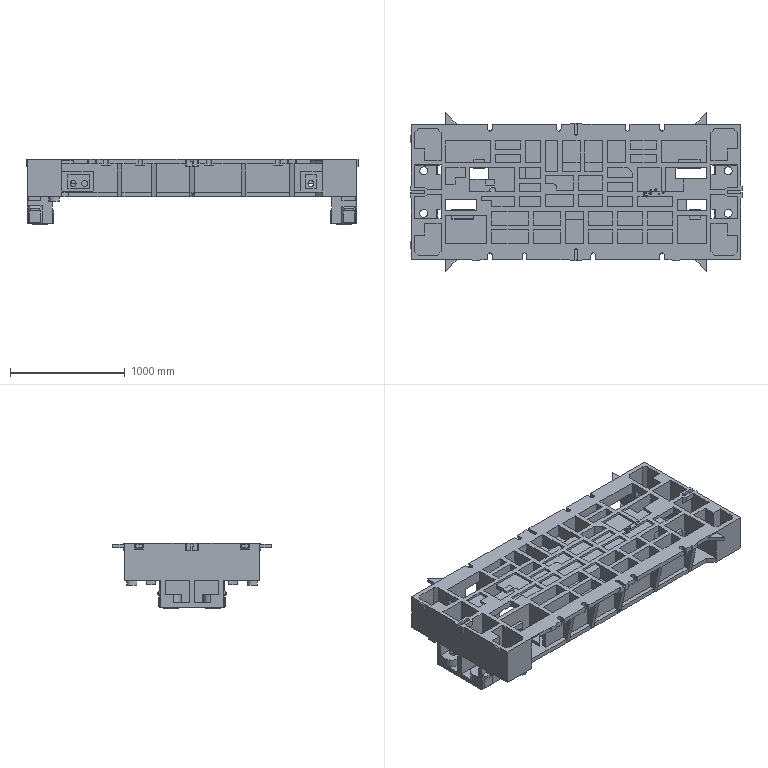Part | NX | features solid 2 | 1 solid | 1165 faces | box 2890 x 1380 x 570 mm | volume 424198456 mm3 | plane 1000 | cylinder 126 | cone 20 | spline 19 | commonest cylinder face diameters 20 x21 50 x16 10 x12 80 x12 32 x9 40 x9